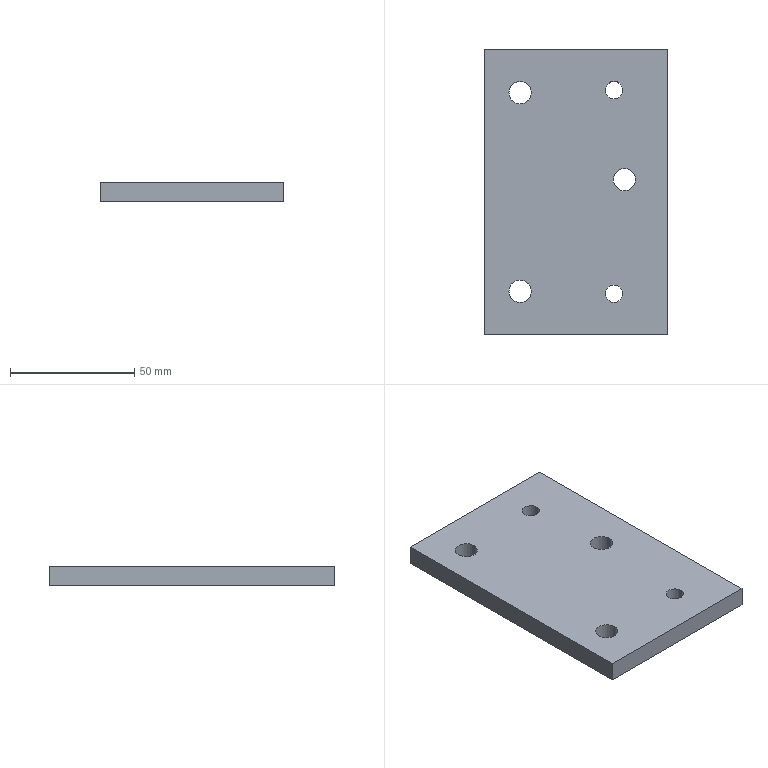Part | 1 solid | 16 faces | box 74 x 115 x 8 mm | volume 65938 mm3 | cylinder 10 | plane 6 | commonest cylinder face diameters 9 x6 7 x4
STEP:
#1=CARTESIAN_POINT('',(0.,0.,0.));
#2=DIRECTION('',(0.,0.,1.));
#3=DIRECTION('',(1.,0.,0.));
#4=AXIS2_PLACEMENT_3D('',#1,#2,#3);
#5=CARTESIAN_POINT('',(-185.5,244.,-105.051));
#6=VERTEX_POINT('',#5);
#7=CARTESIAN_POINT('',(-259.5,244.,-105.051));
#8=VERTEX_POINT('',#7);
#9=CARTESIAN_POINT('',(-185.5,244.,-105.051));
#10=DIRECTION('',(-1.,0.,0.));
#11=VECTOR('',#10,1.);
#12=LINE('',#9,#11);
#13=CARTESIAN_POINT('',(-185.5,244.,-113.051));
#14=DIRECTION('',(0.,1.,0.));
#15=DIRECTION('',(0.,0.,-1.));
#16=AXIS2_PLACEMENT_3D('',#13,#14,#15);
#17=PLANE('',#16);
#18=CARTESIAN_POINT('',(-8.,0.));
#19=DIRECTION('',(0.,1.));
#20=VECTOR('',#19,1.);
#21=LINE('',#18,#20);
#22=(GEOMETRIC_REPRESENTATION_CONTEXT(2)PARAMETRIC_REPRESENTATION_CONTEXT()REPRESENTATION_CONTEXT('',''));
#23=DEFINITIONAL_REPRESENTATION('',(#21),#22);
#24=PCURVE('',#17,#23);
#25=CARTESIAN_POINT('',(-207.188,260.5,-105.051));
#26=DIRECTION('',(0.,0.,1.));
#27=DIRECTION('',(-1.,0.,0.));
#28=AXIS2_PLACEMENT_3D('',#25,#26,#27);
#29=PLANE('',#28);
#30=CARTESIAN_POINT('',(-21.688,16.5));
#31=DIRECTION('',(1.,0.));
#32=VECTOR('',#31,1.);
#33=LINE('',#30,#32);
#34=(GEOMETRIC_REPRESENTATION_CONTEXT(2)PARAMETRIC_REPRESENTATION_CONTEXT()REPRESENTATION_CONTEXT('',''));
#35=DEFINITIONAL_REPRESENTATION('',(#33),#34);
#36=PCURVE('',#29,#35);
#37=SURFACE_CURVE('',#12,(#24,#36),.PCURVE_S1.);
#38=EDGE_CURVE('',#6,#8,#37,.T.);
#39=ORIENTED_EDGE('',*,*,#38,.T.);
#40=CARTESIAN_POINT('',(-259.5,244.,-113.051));
#41=VERTEX_POINT('',#40);
#42=CARTESIAN_POINT('',(-259.5,244.,-113.051));
#43=DIRECTION('',(0.,0.,1.));
#44=VECTOR('',#43,1.);
#45=LINE('',#42,#44);
#46=CARTESIAN_POINT('',(0.,74.));
#47=DIRECTION('',(-1.,0.));
#48=VECTOR('',#47,1.);
#49=LINE('',#46,#48);
#50=(GEOMETRIC_REPRESENTATION_CONTEXT(2)PARAMETRIC_REPRESENTATION_CONTEXT()REPRESENTATION_CONTEXT('',''));
#51=DEFINITIONAL_REPRESENTATION('',(#49),#50);
#52=PCURVE('',#17,#51);
#53=CARTESIAN_POINT('',(-259.5,244.,-113.051));
#54=DIRECTION('',(1.,0.,0.));
#55=DIRECTION('',(0.,0.,1.));
#56=AXIS2_PLACEMENT_3D('',#53,#54,#55);
#57=PLANE('',#56);
#58=CARTESIAN_POINT('',(0.,0.));
#59=DIRECTION('',(1.,0.));
#60=VECTOR('',#59,1.);
#61=LINE('',#58,#60);
#62=(GEOMETRIC_REPRESENTATION_CONTEXT(2)PARAMETRIC_REPRESENTATION_CONTEXT()REPRESENTATION_CONTEXT('',''));
#63=DEFINITIONAL_REPRESENTATION('',(#61),#62);
#64=PCURVE('',#57,#63);
#65=SURFACE_CURVE('',#45,(#52,#64),.PCURVE_S1.);
#66=EDGE_CURVE('',#41,#8,#65,.T.);
#67=ORIENTED_EDGE('',*,*,#66,.F.);
#68=CARTESIAN_POINT('',(-185.5,244.,-113.051));
#69=VERTEX_POINT('',#68);
#70=CARTESIAN_POINT('',(-185.5,244.,-113.051));
#71=DIRECTION('',(-1.,0.,0.));
#72=VECTOR('',#71,1.);
#73=LINE('',#70,#72);
#74=CARTESIAN_POINT('',(0.,0.));
#75=DIRECTION('',(0.,1.));
#76=VECTOR('',#75,1.);
#77=LINE('',#74,#76);
#78=(GEOMETRIC_REPRESENTATION_CONTEXT(2)PARAMETRIC_REPRESENTATION_CONTEXT()REPRESENTATION_CONTEXT('',''));
#79=DEFINITIONAL_REPRESENTATION('',(#77),#78);
#80=PCURVE('',#17,#79);
#81=CARTESIAN_POINT('',(-207.188,260.5,-113.051));
#82=DIRECTION('',(0.,0.,1.));
#83=DIRECTION('',(-1.,0.,0.));
#84=AXIS2_PLACEMENT_3D('',#81,#82,#83);
#85=PLANE('',#84);
#86=CARTESIAN_POINT('',(-21.688,16.5));
#87=DIRECTION('',(1.,0.));
#88=VECTOR('',#87,1.);
#89=LINE('',#86,#88);
#90=(GEOMETRIC_REPRESENTATION_CONTEXT(2)PARAMETRIC_REPRESENTATION_CONTEXT()REPRESENTATION_CONTEXT('',''));
#91=DEFINITIONAL_REPRESENTATION('',(#89),#90);
#92=PCURVE('',#85,#91);
#93=SURFACE_CURVE('',#73,(#80,#92),.PCURVE_S1.);
#94=EDGE_CURVE('',#69,#41,#93,.T.);
#95=ORIENTED_EDGE('',*,*,#94,.F.);
#96=CARTESIAN_POINT('',(-185.5,244.,-113.051));
#97=DIRECTION('',(0.,0.,1.));
#98=VECTOR('',#97,1.);
#99=LINE('',#96,#98);
#100=CARTESIAN_POINT('',(0.,0.));
#101=DIRECTION('',(-1.,0.));
#102=VECTOR('',#101,1.);
#103=LINE('',#100,#102);
#104=(GEOMETRIC_REPRESENTATION_CONTEXT(2)PARAMETRIC_REPRESENTATION_CONTEXT()REPRESENTATION_CONTEXT('',''));
#105=DEFINITIONAL_REPRESENTATION('',(#103),#104);
#106=PCURVE('',#17,#105);
#107=CARTESIAN_POINT('',(-185.5,359.,-113.051));
#108=DIRECTION('',(-1.,0.,0.));
#109=DIRECTION('',(0.,0.,-1.));
#110=AXIS2_PLACEMENT_3D('',#107,#108,#109);
#111=PLANE('',#110);
#112=CARTESIAN_POINT('',(0.,115.));
#113=DIRECTION('',(-1.,0.));
#114=VECTOR('',#113,1.);
#115=LINE('',#112,#114);
#116=(GEOMETRIC_REPRESENTATION_CONTEXT(2)PARAMETRIC_REPRESENTATION_CONTEXT()REPRESENTATION_CONTEXT('',''));
#117=DEFINITIONAL_REPRESENTATION('',(#115),#116);
#118=PCURVE('',#111,#117);
#119=SURFACE_CURVE('',#99,(#106,#118),.PCURVE_S1.);
#120=EDGE_CURVE('',#69,#6,#119,.T.);
#121=ORIENTED_EDGE('',*,*,#120,.T.);
#122=EDGE_LOOP('',(#39,#67,#95,#121));
#123=FACE_BOUND('',#122,.T.);
#124=ADVANCED_FACE('',(#123),#17,.F.);
#125=CARTESIAN_POINT('',(-185.5,359.,-105.051));
#126=VERTEX_POINT('',#125);
#127=CARTESIAN_POINT('',(-185.5,359.,-105.051));
#128=DIRECTION('',(0.,-1.,0.));
#129=VECTOR('',#128,1.);
#130=LINE('',#127,#129);
#131=CARTESIAN_POINT('',(-8.,0.));
#132=DIRECTION('',(0.,1.));
#133=VECTOR('',#132,1.);
#134=LINE('',#131,#133);
#135=(GEOMETRIC_REPRESENTATION_CONTEXT(2)PARAMETRIC_REPRESENTATION_CONTEXT()REPRESENTATION_CONTEXT('',''));
#136=DEFINITIONAL_REPRESENTATION('',(#134),#135);
#137=PCURVE('',#111,#136);
#138=CARTESIAN_POINT('',(-21.688,-98.5));
#139=DIRECTION('',(0.,1.));
#140=VECTOR('',#139,1.);
#141=LINE('',#138,#140);
#142=(GEOMETRIC_REPRESENTATION_CONTEXT(2)PARAMETRIC_REPRESENTATION_CONTEXT()REPRESENTATION_CONTEXT('',''));
#143=DEFINITIONAL_REPRESENTATION('',(#141),#142);
#144=PCURVE('',#29,#143);
#145=SURFACE_CURVE('',#130,(#137,#144),.PCURVE_S1.);
#146=EDGE_CURVE('',#126,#6,#145,.T.);
#147=ORIENTED_EDGE('',*,*,#146,.T.);
#148=ORIENTED_EDGE('',*,*,#120,.F.);
#149=CARTESIAN_POINT('',(-185.5,359.,-113.051));
#150=VERTEX_POINT('',#149);
#151=CARTESIAN_POINT('',(-185.5,359.,-113.051));
#152=DIRECTION('',(0.,-1.,0.));
#153=VECTOR('',#152,1.);
#154=LINE('',#151,#153);
#155=CARTESIAN_POINT('',(0.,0.));
#156=DIRECTION('',(0.,1.));
#157=VECTOR('',#156,1.);
#158=LINE('',#155,#157);
#159=(GEOMETRIC_REPRESENTATION_CONTEXT(2)PARAMETRIC_REPRESENTATION_CONTEXT()REPRESENTATION_CONTEXT('',''));
#160=DEFINITIONAL_REPRESENTATION('',(#158),#159);
#161=PCURVE('',#111,#160);
#162=CARTESIAN_POINT('',(-21.688,-98.5));
#163=DIRECTION('',(0.,1.));
#164=VECTOR('',#163,1.);
#165=LINE('',#162,#164);
#166=(GEOMETRIC_REPRESENTATION_CONTEXT(2)PARAMETRIC_REPRESENTATION_CONTEXT()REPRESENTATION_CONTEXT('',''));
#167=DEFINITIONAL_REPRESENTATION('',(#165),#166);
#168=PCURVE('',#85,#167);
#169=SURFACE_CURVE('',#154,(#161,#168),.PCURVE_S1.);
#170=EDGE_CURVE('',#150,#69,#169,.T.);
#171=ORIENTED_EDGE('',*,*,#170,.F.);
#172=CARTESIAN_POINT('',(-185.5,359.,-113.051));
#173=DIRECTION('',(0.,0.,1.));
#174=VECTOR('',#173,1.);
#175=LINE('',#172,#174);
#176=CARTESIAN_POINT('',(0.,0.));
#177=DIRECTION('',(-1.,0.));
#178=VECTOR('',#177,1.);
#179=LINE('',#176,#178);
#180=(GEOMETRIC_REPRESENTATION_CONTEXT(2)PARAMETRIC_REPRESENTATION_CONTEXT()REPRESENTATION_CONTEXT('',''));
#181=DEFINITIONAL_REPRESENTATION('',(#179),#180);
#182=PCURVE('',#111,#181);
#183=CARTESIAN_POINT('',(-259.5,359.,-113.051));
#184=DIRECTION('',(0.,-1.,0.));
#185=DIRECTION('',(0.,0.,1.));
#186=AXIS2_PLACEMENT_3D('',#183,#184,#185);
#187=PLANE('',#186);
#188=CARTESIAN_POINT('',(0.,-74.));
#189=DIRECTION('',(1.,0.));
#190=VECTOR('',#189,1.);
#191=LINE('',#188,#190);
#192=(GEOMETRIC_REPRESENTATION_CONTEXT(2)PARAMETRIC_REPRESENTATION_CONTEXT()REPRESENTATION_CONTEXT('',''));
#193=DEFINITIONAL_REPRESENTATION('',(#191),#192);
#194=PCURVE('',#187,#193);
#195=SURFACE_CURVE('',#175,(#182,#194),.PCURVE_S1.);
#196=EDGE_CURVE('',#150,#126,#195,.T.);
#197=ORIENTED_EDGE('',*,*,#196,.T.);
#198=EDGE_LOOP('',(#147,#148,#171,#197));
#199=FACE_BOUND('',#198,.T.);
#200=ADVANCED_FACE('',(#199),#111,.F.);
#201=CARTESIAN_POINT('',(-259.5,359.,-105.051));
#202=VERTEX_POINT('',#201);
#203=CARTESIAN_POINT('',(-259.5,359.,-105.051));
#204=DIRECTION('',(1.,0.,0.));
#205=VECTOR('',#204,1.);
#206=LINE('',#203,#205);
#207=CARTESIAN_POINT('',(8.,0.));
#208=DIRECTION('',(0.,-1.));
#209=VECTOR('',#208,1.);
#210=LINE('',#207,#209);
#211=(GEOMETRIC_REPRESENTATION_CONTEXT(2)PARAMETRIC_REPRESENTATION_CONTEXT()REPRESENTATION_CONTEXT('',''));
#212=DEFINITIONAL_REPRESENTATION('',(#210),#211);
#213=PCURVE('',#187,#212);
#214=CARTESIAN_POINT('',(52.312,-98.5));
#215=DIRECTION('',(-1.,0.));
#216=VECTOR('',#215,1.);
#217=LINE('',#214,#216);
#218=(GEOMETRIC_REPRESENTATION_CONTEXT(2)PARAMETRIC_REPRESENTATION_CONTEXT()REPRESENTATION_CONTEXT('',''));
#219=DEFINITIONAL_REPRESENTATION('',(#217),#218);
#220=PCURVE('',#29,#219);
#221=SURFACE_CURVE('',#206,(#213,#220),.PCURVE_S1.);
#222=EDGE_CURVE('',#202,#126,#221,.T.);
#223=ORIENTED_EDGE('',*,*,#222,.T.);
#224=ORIENTED_EDGE('',*,*,#196,.F.);
#225=CARTESIAN_POINT('',(-259.5,359.,-113.051));
#226=VERTEX_POINT('',#225);
#227=CARTESIAN_POINT('',(-259.5,359.,-113.051));
#228=DIRECTION('',(1.,0.,0.));
#229=VECTOR('',#228,1.);
#230=LINE('',#227,#229);
#231=CARTESIAN_POINT('',(0.,0.));
#232=DIRECTION('',(0.,-1.));
#233=VECTOR('',#232,1.);
#234=LINE('',#231,#233);
#235=(GEOMETRIC_REPRESENTATION_CONTEXT(2)PARAMETRIC_REPRESENTATION_CONTEXT()REPRESENTATION_CONTEXT('',''));
#236=DEFINITIONAL_REPRESENTATION('',(#234),#235);
#237=PCURVE('',#187,#236);
#238=CARTESIAN_POINT('',(52.312,-98.5));
#239=DIRECTION('',(-1.,0.));
#240=VECTOR('',#239,1.);
#241=LINE('',#238,#240);
#242=(GEOMETRIC_REPRESENTATION_CONTEXT(2)PARAMETRIC_REPRESENTATION_CONTEXT()REPRESENTATION_CONTEXT('',''));
#243=DEFINITIONAL_REPRESENTATION('',(#241),#242);
#244=PCURVE('',#85,#243);
#245=SURFACE_CURVE('',#230,(#237,#244),.PCURVE_S1.);
#246=EDGE_CURVE('',#226,#150,#245,.T.);
#247=ORIENTED_EDGE('',*,*,#246,.F.);
#248=CARTESIAN_POINT('',(-259.5,359.,-113.051));
#249=DIRECTION('',(0.,0.,1.));
#250=VECTOR('',#249,1.);
#251=LINE('',#248,#250);
#252=CARTESIAN_POINT('',(0.,0.));
#253=DIRECTION('',(1.,0.));
#254=VECTOR('',#253,1.);
#255=LINE('',#252,#254);
#256=(GEOMETRIC_REPRESENTATION_CONTEXT(2)PARAMETRIC_REPRESENTATION_CONTEXT()REPRESENTATION_CONTEXT('',''));
#257=DEFINITIONAL_REPRESENTATION('',(#255),#256);
#258=PCURVE('',#187,#257);
#259=CARTESIAN_POINT('',(0.,-115.));
#260=DIRECTION('',(1.,0.));
#261=VECTOR('',#260,1.);
#262=LINE('',#259,#261);
#263=(GEOMETRIC_REPRESENTATION_CONTEXT(2)PARAMETRIC_REPRESENTATION_CONTEXT()REPRESENTATION_CONTEXT('',''));
#264=DEFINITIONAL_REPRESENTATION('',(#262),#263);
#265=PCURVE('',#57,#264);
#266=SURFACE_CURVE('',#251,(#258,#265),.PCURVE_S1.);
#267=EDGE_CURVE('',#226,#202,#266,.T.);
#268=ORIENTED_EDGE('',*,*,#267,.T.);
#269=EDGE_LOOP('',(#223,#224,#247,#268));
#270=FACE_BOUND('',#269,.T.);
#271=ADVANCED_FACE('',(#270),#187,.F.);
#272=CARTESIAN_POINT('',(-259.5,244.,-105.051));
#273=DIRECTION('',(0.,1.,0.));
#274=VECTOR('',#273,1.);
#275=LINE('',#272,#274);
#276=CARTESIAN_POINT('',(8.,0.));
#277=DIRECTION('',(0.,-1.));
#278=VECTOR('',#277,1.);
#279=LINE('',#276,#278);
#280=(GEOMETRIC_REPRESENTATION_CONTEXT(2)PARAMETRIC_REPRESENTATION_CONTEXT()REPRESENTATION_CONTEXT('',''));
#281=DEFINITIONAL_REPRESENTATION('',(#279),#280);
#282=PCURVE('',#57,#281);
#283=CARTESIAN_POINT('',(52.312,16.5));
#284=DIRECTION('',(0.,-1.));
#285=VECTOR('',#284,1.);
#286=LINE('',#283,#285);
#287=(GEOMETRIC_REPRESENTATION_CONTEXT(2)PARAMETRIC_REPRESENTATION_CONTEXT()REPRESENTATION_CONTEXT('',''));
#288=DEFINITIONAL_REPRESENTATION('',(#286),#287);
#289=PCURVE('',#29,#288);
#290=SURFACE_CURVE('',#275,(#282,#289),.PCURVE_S1.);
#291=EDGE_CURVE('',#8,#202,#290,.T.);
#292=ORIENTED_EDGE('',*,*,#291,.T.);
#293=ORIENTED_EDGE('',*,*,#267,.F.);
#294=CARTESIAN_POINT('',(-259.5,244.,-113.051));
#295=DIRECTION('',(0.,1.,0.));
#296=VECTOR('',#295,1.);
#297=LINE('',#294,#296);
#298=CARTESIAN_POINT('',(0.,0.));
#299=DIRECTION('',(0.,-1.));
#300=VECTOR('',#299,1.);
#301=LINE('',#298,#300);
#302=(GEOMETRIC_REPRESENTATION_CONTEXT(2)PARAMETRIC_REPRESENTATION_CONTEXT()REPRESENTATION_CONTEXT('',''));
#303=DEFINITIONAL_REPRESENTATION('',(#301),#302);
#304=PCURVE('',#57,#303);
#305=CARTESIAN_POINT('',(52.312,16.5));
#306=DIRECTION('',(0.,-1.));
#307=VECTOR('',#306,1.);
#308=LINE('',#305,#307);
#309=(GEOMETRIC_REPRESENTATION_CONTEXT(2)PARAMETRIC_REPRESENTATION_CONTEXT()REPRESENTATION_CONTEXT('',''));
#310=DEFINITIONAL_REPRESENTATION('',(#308),#309);
#311=PCURVE('',#85,#310);
#312=SURFACE_CURVE('',#297,(#304,#311),.PCURVE_S1.);
#313=EDGE_CURVE('',#41,#226,#312,.T.);
#314=ORIENTED_EDGE('',*,*,#313,.F.);
#315=ORIENTED_EDGE('',*,*,#66,.T.);
#316=EDGE_LOOP('',(#292,#293,#314,#315));
#317=FACE_BOUND('',#316,.T.);
#318=ADVANCED_FACE('',(#317),#57,.F.);
#319=ORIENTED_EDGE('',*,*,#94,.T.);
#320=ORIENTED_EDGE('',*,*,#313,.T.);
#321=ORIENTED_EDGE('',*,*,#246,.T.);
#322=ORIENTED_EDGE('',*,*,#170,.T.);
#323=EDGE_LOOP('',(#319,#320,#321,#322));
#324=FACE_BOUND('',#323,.T.);
#325=CARTESIAN_POINT('',(-210.688,260.5,-113.051));
#326=VERTEX_POINT('',#325);
#327=CARTESIAN_POINT('',(-203.688,260.5,-113.051));
#328=VERTEX_POINT('',#327);
#329=CARTESIAN_POINT('',(-207.188,260.5,-113.051));
#330=DIRECTION('',(0.,0.,1.));
#331=DIRECTION('',(-1.,0.,0.));
#332=AXIS2_PLACEMENT_3D('',#329,#330,#331);
#333=CIRCLE('',#332,3.5);
#334=CARTESIAN_POINT('',(0.,0.));
#335=DIRECTION('',(1.,0.));
#336=AXIS2_PLACEMENT_2D('',#334,#335);
#337=CIRCLE('',#336,3.5);
#338=(GEOMETRIC_REPRESENTATION_CONTEXT(2)PARAMETRIC_REPRESENTATION_CONTEXT()REPRESENTATION_CONTEXT('',''));
#339=DEFINITIONAL_REPRESENTATION('',(#337),#338);
#340=PCURVE('',#85,#339);
#341=CARTESIAN_POINT('',(-207.188,260.5,-113.051));
#342=DIRECTION('',(0.,0.,1.));
#343=DIRECTION('',(0.,1.,0.));
#344=AXIS2_PLACEMENT_3D('',#341,#342,#343);
#345=CYLINDRICAL_SURFACE('',#344,3.5);
#346=CARTESIAN_POINT('',(1.571,0.));
#347=DIRECTION('',(1.,0.));
#348=VECTOR('',#347,1.);
#349=LINE('',#346,#348);
#350=(GEOMETRIC_REPRESENTATION_CONTEXT(2)PARAMETRIC_REPRESENTATION_CONTEXT()REPRESENTATION_CONTEXT('',''));
#351=DEFINITIONAL_REPRESENTATION('',(#349),#350);
#352=PCURVE('',#345,#351);
#353=SURFACE_CURVE('',#333,(#340,#352),.PCURVE_S1.);
#354=EDGE_CURVE('',#326,#328,#353,.T.);
#355=ORIENTED_EDGE('',*,*,#354,.T.);
#356=CARTESIAN_POINT('',(-207.188,260.5,-113.051));
#357=DIRECTION('',(0.,0.,1.));
#358=DIRECTION('',(-1.,0.,0.));
#359=AXIS2_PLACEMENT_3D('',#356,#357,#358);
#360=CIRCLE('',#359,3.5);
#361=CARTESIAN_POINT('',(0.,0.));
#362=DIRECTION('',(1.,0.));
#363=AXIS2_PLACEMENT_2D('',#361,#362);
#364=CIRCLE('',#363,3.5);
#365=(GEOMETRIC_REPRESENTATION_CONTEXT(2)PARAMETRIC_REPRESENTATION_CONTEXT()REPRESENTATION_CONTEXT('',''));
#366=DEFINITIONAL_REPRESENTATION('',(#364),#365);
#367=PCURVE('',#85,#366);
#368=CARTESIAN_POINT('',(-207.188,260.5,-113.051));
#369=DIRECTION('',(0.,0.,1.));
#370=DIRECTION('',(0.,-1.,0.));
#371=AXIS2_PLACEMENT_3D('',#368,#369,#370);
#372=CYLINDRICAL_SURFACE('',#371,3.5);
#373=CARTESIAN_POINT('',(-1.571,0.));
#374=DIRECTION('',(1.,0.));
#375=VECTOR('',#374,1.);
#376=LINE('',#373,#375);
#377=(GEOMETRIC_REPRESENTATION_CONTEXT(2)PARAMETRIC_REPRESENTATION_CONTEXT()REPRESENTATION_CONTEXT('',''));
#378=DEFINITIONAL_REPRESENTATION('',(#376),#377);
#379=PCURVE('',#372,#378);
#380=SURFACE_CURVE('',#360,(#367,#379),.PCURVE_S1.);
#381=EDGE_CURVE('',#328,#326,#380,.T.);
#382=ORIENTED_EDGE('',*,*,#381,.T.);
#383=EDGE_LOOP('',(#355,#382));
#384=FACE_BOUND('',#383,.T.);
#385=CARTESIAN_POINT('',(-207.5,306.5,-113.051));
#386=VERTEX_POINT('',#385);
#387=CARTESIAN_POINT('',(-198.5,306.5,-113.051));
#388=VERTEX_POINT('',#387);
#389=CARTESIAN_POINT('',(-203.,306.5,-113.051));
#390=DIRECTION('',(0.,0.,1.));
#391=DIRECTION('',(-1.,0.,0.));
#392=AXIS2_PLACEMENT_3D('',#389,#390,#391);
#393=CIRCLE('',#392,4.5);
#394=CARTESIAN_POINT('',(-4.188,-46.));
#395=DIRECTION('',(1.,0.));
#396=AXIS2_PLACEMENT_2D('',#394,#395);
#397=CIRCLE('',#396,4.5);
#398=(GEOMETRIC_REPRESENTATION_CONTEXT(2)PARAMETRIC_REPRESENTATION_CONTEXT()REPRESENTATION_CONTEXT('',''));
#399=DEFINITIONAL_REPRESENTATION('',(#397),#398);
#400=PCURVE('',#85,#399);
#401=CARTESIAN_POINT('',(-203.,306.5,-113.051));
#402=DIRECTION('',(0.,0.,1.));
#403=DIRECTION('',(0.,1.,0.));
#404=AXIS2_PLACEMENT_3D('',#401,#402,#403);
#405=CYLINDRICAL_SURFACE('',#404,4.5);
#406=CARTESIAN_POINT('',(1.571,0.));
#407=DIRECTION('',(1.,0.));
#408=VECTOR('',#407,1.);
#409=LINE('',#406,#408);
#410=(GEOMETRIC_REPRESENTATION_CONTEXT(2)PARAMETRIC_REPRESENTATION_CONTEXT()REPRESENTATION_CONTEXT('',''));
#411=DEFINITIONAL_REPRESENTATION('',(#409),#410);
#412=PCURVE('',#405,#411);
#413=SURFACE_CURVE('',#393,(#400,#412),.PCURVE_S1.);
#414=EDGE_CURVE('',#386,#388,#413,.T.);
#415=ORIENTED_EDGE('',*,*,#414,.T.);
#416=CARTESIAN_POINT('',(-203.,306.5,-113.051));
#417=DIRECTION('',(0.,0.,1.));
#418=DIRECTION('',(-1.,0.,0.));
#419=AXIS2_PLACEMENT_3D('',#416,#417,#418);
#420=CIRCLE('',#419,4.5);
#421=CARTESIAN_POINT('',(-4.188,-46.));
#422=DIRECTION('',(1.,0.));
#423=AXIS2_PLACEMENT_2D('',#421,#422);
#424=CIRCLE('',#423,4.5);
#425=(GEOMETRIC_REPRESENTATION_CONTEXT(2)PARAMETRIC_REPRESENTATION_CONTEXT()REPRESENTATION_CONTEXT('',''));
#426=DEFINITIONAL_REPRESENTATION('',(#424),#425);
#427=PCURVE('',#85,#426);
#428=CARTESIAN_POINT('',(-203.,306.5,-113.051));
#429=DIRECTION('',(0.,0.,1.));
#430=DIRECTION('',(0.,-1.,0.));
#431=AXIS2_PLACEMENT_3D('',#428,#429,#430);
#432=CYLINDRICAL_SURFACE('',#431,4.5);
#433=CARTESIAN_POINT('',(-1.571,0.));
#434=DIRECTION('',(1.,0.));
#435=VECTOR('',#434,1.);
#436=LINE('',#433,#435);
#437=(GEOMETRIC_REPRESENTATION_CONTEXT(2)PARAMETRIC_REPRESENTATION_CONTEXT()REPRESENTATION_CONTEXT('',''));
#438=DEFINITIONAL_REPRESENTATION('',(#436),#437);
#439=PCURVE('',#432,#438);
#440=SURFACE_CURVE('',#420,(#427,#439),.PCURVE_S1.);
#441=EDGE_CURVE('',#388,#386,#440,.T.);
#442=ORIENTED_EDGE('',*,*,#441,.T.);
#443=EDGE_LOOP('',(#415,#442));
#444=FACE_BOUND('',#443,.T.);
#445=CARTESIAN_POINT('',(-249.5,261.5,-113.051));
#446=VERTEX_POINT('',#445);
#447=CARTESIAN_POINT('',(-240.5,261.5,-113.051));
#448=VERTEX_POINT('',#447);
#449=CARTESIAN_POINT('',(-245.,261.5,-113.051));
#450=DIRECTION('',(0.,0.,1.));
#451=DIRECTION('',(-1.,0.,0.));
#452=AXIS2_PLACEMENT_3D('',#449,#450,#451);
#453=CIRCLE('',#452,4.5);
#454=CARTESIAN_POINT('',(37.812,-0.9999));
#455=DIRECTION('',(1.,0.));
#456=AXIS2_PLACEMENT_2D('',#454,#455);
#457=CIRCLE('',#456,4.5);
#458=(GEOMETRIC_REPRESENTATION_CONTEXT(2)PARAMETRIC_REPRESENTATION_CONTEXT()REPRESENTATION_CONTEXT('',''));
#459=DEFINITIONAL_REPRESENTATION('',(#457),#458);
#460=PCURVE('',#85,#459);
#461=CARTESIAN_POINT('',(-245.,261.5,-113.051));
#462=DIRECTION('',(0.,0.,1.));
#463=DIRECTION('',(0.,1.,0.));
#464=AXIS2_PLACEMENT_3D('',#461,#462,#463);
#465=CYLINDRICAL_SURFACE('',#464,4.5);
#466=CARTESIAN_POINT('',(1.571,0.));
#467=DIRECTION('',(1.,0.));
#468=VECTOR('',#467,1.);
#469=LINE('',#466,#468);
#470=(GEOMETRIC_REPRESENTATION_CONTEXT(2)PARAMETRIC_REPRESENTATION_CONTEXT()REPRESENTATION_CONTEXT('',''));
#471=DEFINITIONAL_REPRESENTATION('',(#469),#470);
#472=PCURVE('',#465,#471);
#473=SURFACE_CURVE('',#453,(#460,#472),.PCURVE_S1.);
#474=EDGE_CURVE('',#446,#448,#473,.T.);
#475=ORIENTED_EDGE('',*,*,#474,.T.);
#476=CARTESIAN_POINT('',(-245.,261.5,-113.051));
#477=DIRECTION('',(0.,0.,1.));
#478=DIRECTION('',(-1.,0.,0.));
#479=AXIS2_PLACEMENT_3D('',#476,#477,#478);
#480=CIRCLE('',#479,4.5);
#481=CARTESIAN_POINT('',(37.812,-0.9999));
#482=DIRECTION('',(1.,0.));
#483=AXIS2_PLACEMENT_2D('',#481,#482);
#484=CIRCLE('',#483,4.5);
#485=(GEOMETRIC_REPRESENTATION_CONTEXT(2)PARAMETRIC_REPRESENTATION_CONTEXT()REPRESENTATION_CONTEXT('',''));
#486=DEFINITIONAL_REPRESENTATION('',(#484),#485);
#487=PCURVE('',#85,#486);
#488=CARTESIAN_POINT('',(-245.,261.5,-113.051));
#489=DIRECTION('',(0.,0.,1.));
#490=DIRECTION('',(0.,-1.,0.));
#491=AXIS2_PLACEMENT_3D('',#488,#489,#490);
#492=CYLINDRICAL_SURFACE('',#491,4.5);
#493=CARTESIAN_POINT('',(-1.571,0.));
#494=DIRECTION('',(1.,0.));
#495=VECTOR('',#494,1.);
#496=LINE('',#493,#495);
#497=(GEOMETRIC_REPRESENTATION_CONTEXT(2)PARAMETRIC_REPRESENTATION_CONTEXT()REPRESENTATION_CONTEXT('',''));
#498=DEFINITIONAL_REPRESENTATION('',(#496),#497);
#499=PCURVE('',#492,#498);
#500=SURFACE_CURVE('',#480,(#487,#499),.PCURVE_S1.);
#501=EDGE_CURVE('',#448,#446,#500,.T.);
#502=ORIENTED_EDGE('',*,*,#501,.T.);
#503=EDGE_LOOP('',(#475,#502));
#504=FACE_BOUND('',#503,.T.);
#505=CARTESIAN_POINT('',(-210.688,342.5,-113.051));
#506=VERTEX_POINT('',#505);
#507=CARTESIAN_POINT('',(-203.688,342.5,-113.051));
#508=VERTEX_POINT('',#507);
#509=CARTESIAN_POINT('',(-207.188,342.5,-113.051));
#510=DIRECTION('',(0.,0.,1.));
#511=DIRECTION('',(-1.,0.,0.));
#512=AXIS2_PLACEMENT_3D('',#509,#510,#511);
#513=CIRCLE('',#512,3.5);
#514=CARTESIAN_POINT('',(0.,-82.));
#515=DIRECTION('',(1.,0.));
#516=AXIS2_PLACEMENT_2D('',#514,#515);
#517=CIRCLE('',#516,3.5);
#518=(GEOMETRIC_REPRESENTATION_CONTEXT(2)PARAMETRIC_REPRESENTATION_CONTEXT()REPRESENTATION_CONTEXT('',''));
#519=DEFINITIONAL_REPRESENTATION('',(#517),#518);
#520=PCURVE('',#85,#519);
#521=CARTESIAN_POINT('',(-207.188,342.5,-113.051));
#522=DIRECTION('',(0.,0.,1.));
#523=DIRECTION('',(0.,1.,0.));
#524=AXIS2_PLACEMENT_3D('',#521,#522,#523);
#525=CYLINDRICAL_SURFACE('',#524,3.5);
#526=CARTESIAN_POINT('',(1.571,0.));
#527=DIRECTION('',(1.,0.));
#528=VECTOR('',#527,1.);
#529=LINE('',#526,#528);
#530=(GEOMETRIC_REPRESENTATION_CONTEXT(2)PARAMETRIC_REPRESENTATION_CONTEXT()REPRESENTATION_CONTEXT('',''));
#531=DEFINITIONAL_REPRESENTATION('',(#529),#530);
#532=PCURVE('',#525,#531);
#533=SURFACE_CURVE('',#513,(#520,#532),.PCURVE_S1.);
#534=EDGE_CURVE('',#506,#508,#533,.T.);
#535=ORIENTED_EDGE('',*,*,#534,.T.);
#536=CARTESIAN_POINT('',(-207.188,342.5,-113.051));
#537=DIRECTION('',(0.,0.,1.));
#538=DIRECTION('',(-1.,0.,0.));
#539=AXIS2_PLACEMENT_3D('',#536,#537,#538);
#540=CIRCLE('',#539,3.5);
#541=CARTESIAN_POINT('',(0.,-82.));
#542=DIRECTION('',(1.,0.));
#543=AXIS2_PLACEMENT_2D('',#541,#542);
#544=CIRCLE('',#543,3.5);
#545=(GEOMETRIC_REPRESENTATION_CONTEXT(2)PARAMETRIC_REPRESENTATION_CONTEXT()REPRESENTATION_CONTEXT('',''));
#546=DEFINITIONAL_REPRESENTATION('',(#544),#545);
#547=PCURVE('',#85,#546);
#548=CARTESIAN_POINT('',(-207.188,342.5,-113.051));
#549=DIRECTION('',(0.,0.,1.));
#550=DIRECTION('',(0.,-1.,0.));
#551=AXIS2_PLACEMENT_3D('',#548,#549,#550);
#552=CYLINDRICAL_SURFACE('',#551,3.5);
#553=CARTESIAN_POINT('',(-1.571,0.));
#554=DIRECTION('',(1.,0.));
#555=VECTOR('',#554,1.);
#556=LINE('',#553,#555);
#557=(GEOMETRIC_REPRESENTATION_CONTEXT(2)PARAMETRIC_REPRESENTATION_CONTEXT()REPRESENTATION_CONTEXT('',''));
#558=DEFINITIONAL_REPRESENTATION('',(#556),#557);
#559=PCURVE('',#552,#558);
#560=SURFACE_CURVE('',#540,(#547,#559),.PCURVE_S1.);
#561=EDGE_CURVE('',#508,#506,#560,.T.);
#562=ORIENTED_EDGE('',*,*,#561,.T.);
#563=EDGE_LOOP('',(#535,#562));
#564=FACE_BOUND('',#563,.T.);
#565=CARTESIAN_POINT('',(-249.5,341.5,-113.051));
#566=VERTEX_POINT('',#565);
#567=CARTESIAN_POINT('',(-240.5,341.5,-113.051));
#568=VERTEX_POINT('',#567);
#569=CARTESIAN_POINT('',(-245.,341.5,-113.051));
#570=DIRECTION('',(0.,0.,1.));
#571=DIRECTION('',(-1.,0.,0.));
#572=AXIS2_PLACEMENT_3D('',#569,#570,#571);
#573=CIRCLE('',#572,4.5);
#574=CARTESIAN_POINT('',(37.812,-81.));
#575=DIRECTION('',(1.,0.));
#576=AXIS2_PLACEMENT_2D('',#574,#575);
#577=CIRCLE('',#576,4.5);
#578=(GEOMETRIC_REPRESENTATION_CONTEXT(2)PARAMETRIC_REPRESENTATION_CONTEXT()REPRESENTATION_CONTEXT('',''));
#579=DEFINITIONAL_REPRESENTATION('',(#577),#578);
#580=PCURVE('',#85,#579);
#581=CARTESIAN_POINT('',(-245.,341.5,-113.051));
#582=DIRECTION('',(0.,0.,1.));
#583=DIRECTION('',(0.,1.,0.));
#584=AXIS2_PLACEMENT_3D('',#581,#582,#583);
#585=CYLINDRICAL_SURFACE('',#584,4.5);
#586=CARTESIAN_POINT('',(1.571,0.));
#587=DIRECTION('',(1.,0.));
#588=VECTOR('',#587,1.);
#589=LINE('',#586,#588);
#590=(GEOMETRIC_REPRESENTATION_CONTEXT(2)PARAMETRIC_REPRESENTATION_CONTEXT()REPRESENTATION_CONTEXT('',''));
#591=DEFINITIONAL_REPRESENTATION('',(#589),#590);
#592=PCURVE('',#585,#591);
#593=SURFACE_CURVE('',#573,(#580,#592),.PCURVE_S1.);
#594=EDGE_CURVE('',#566,#568,#593,.T.);
#595=ORIENTED_EDGE('',*,*,#594,.T.);
#596=CARTESIAN_POINT('',(-245.,341.5,-113.051));
#597=DIRECTION('',(0.,0.,1.));
#598=DIRECTION('',(-1.,0.,0.));
#599=AXIS2_PLACEMENT_3D('',#596,#597,#598);
#600=CIRCLE('',#599,4.5);
#601=CARTESIAN_POINT('',(37.812,-81.));
#602=DIRECTION('',(1.,0.));
#603=AXIS2_PLACEMENT_2D('',#601,#602);
#604=CIRCLE('',#603,4.5);
#605=(GEOMETRIC_REPRESENTATION_CONTEXT(2)PARAMETRIC_REPRESENTATION_CONTEXT()REPRESENTATION_CONTEXT('',''));
#606=DEFINITIONAL_REPRESENTATION('',(#604),#605);
#607=PCURVE('',#85,#606);
#608=CARTESIAN_POINT('',(-245.,341.5,-113.051));
#609=DIRECTION('',(0.,0.,1.));
#610=DIRECTION('',(0.,-1.,0.));
#611=AXIS2_PLACEMENT_3D('',#608,#609,#610);
#612=CYLINDRICAL_SURFACE('',#611,4.5);
#613=CARTESIAN_POINT('',(-1.571,0.));
#614=DIRECTION('',(1.,0.));
#615=VECTOR('',#614,1.);
#616=LINE('',#613,#615);
#617=(GEOMETRIC_REPRESENTATION_CONTEXT(2)PARAMETRIC_REPRESENTATION_CONTEXT()REPRESENTATION_CONTEXT('',''));
#618=DEFINITIONAL_REPRESENTATION('',(#616),#617);
#619=PCURVE('',#612,#618);
#620=SURFACE_CURVE('',#600,(#607,#619),.PCURVE_S1.);
#621=EDGE_CURVE('',#568,#566,#620,.T.);
#622=ORIENTED_EDGE('',*,*,#621,.T.);
#623=EDGE_LOOP('',(#595,#622));
#624=FACE_BOUND('',#623,.T.);
#625=ADVANCED_FACE('',(#324,#384,#444,#504,#564,#624),#85,.F.);
#626=ORIENTED_EDGE('',*,*,#621,.T.);
#627=CARTESIAN_POINT('',(-249.5,341.5,-105.051));
#628=VERTEX_POINT('',#627);
#629=CARTESIAN_POINT('',(-249.5,341.5,-113.051));
#630=DIRECTION('',(0.,0.,1.));
#631=VECTOR('',#630,1.);
#632=LINE('',#629,#631);
#633=CARTESIAN_POINT('',(4.712,0.));
#634=DIRECTION('',(0.,1.));
#635=VECTOR('',#634,1.);
#636=LINE('',#633,#635);
#637=(GEOMETRIC_REPRESENTATION_CONTEXT(2)PARAMETRIC_REPRESENTATION_CONTEXT()REPRESENTATION_CONTEXT('',''));
#638=DEFINITIONAL_REPRESENTATION('',(#636),#637);
#639=PCURVE('',#612,#638);
#640=CARTESIAN_POINT('',(1.571,0.));
#641=DIRECTION('',(0.,1.));
#642=VECTOR('',#641,1.);
#643=LINE('',#640,#642);
#644=(GEOMETRIC_REPRESENTATION_CONTEXT(2)PARAMETRIC_REPRESENTATION_CONTEXT()REPRESENTATION_CONTEXT('',''));
#645=DEFINITIONAL_REPRESENTATION('',(#643),#644);
#646=PCURVE('',#585,#645);
#647=SURFACE_CURVE('',#632,(#639,#646),.PCURVE_S1.);
#648=EDGE_CURVE('',#566,#628,#647,.T.);
#649=ORIENTED_EDGE('',*,*,#648,.T.);
#650=CARTESIAN_POINT('',(-240.5,341.5,-105.051));
#651=VERTEX_POINT('',#650);
#652=CARTESIAN_POINT('',(-245.,341.5,-105.051));
#653=DIRECTION('',(0.,0.,1.));
#654=DIRECTION('',(-1.,0.,0.));
#655=AXIS2_PLACEMENT_3D('',#652,#653,#654);
#656=CIRCLE('',#655,4.5);
#657=CARTESIAN_POINT('',(-1.571,8.));
#658=DIRECTION('',(1.,0.));
#659=VECTOR('',#658,1.);
#660=LINE('',#657,#659);
#661=(GEOMETRIC_REPRESENTATION_CONTEXT(2)PARAMETRIC_REPRESENTATION_CONTEXT()REPRESENTATION_CONTEXT('',''));
#662=DEFINITIONAL_REPRESENTATION('',(#660),#661);
#663=PCURVE('',#612,#662);
#664=CARTESIAN_POINT('',(37.812,-81.));
#665=DIRECTION('',(1.,0.));
#666=AXIS2_PLACEMENT_2D('',#664,#665);
#667=CIRCLE('',#666,4.5);
#668=(GEOMETRIC_REPRESENTATION_CONTEXT(2)PARAMETRIC_REPRESENTATION_CONTEXT()REPRESENTATION_CONTEXT('',''));
#669=DEFINITIONAL_REPRESENTATION('',(#667),#668);
#670=PCURVE('',#29,#669);
#671=SURFACE_CURVE('',#656,(#663,#670),.PCURVE_S1.);
#672=EDGE_CURVE('',#651,#628,#671,.T.);
#673=ORIENTED_EDGE('',*,*,#672,.F.);
#674=CARTESIAN_POINT('',(-240.5,341.5,-113.051));
#675=DIRECTION('',(0.,0.,1.));
#676=VECTOR('',#675,1.);
#677=LINE('',#674,#676);
#678=CARTESIAN_POINT('',(1.571,0.));
#679=DIRECTION('',(0.,1.));
#680=VECTOR('',#679,1.);
#681=LINE('',#678,#680);
#682=(GEOMETRIC_REPRESENTATION_CONTEXT(2)PARAMETRIC_REPRESENTATION_CONTEXT()REPRESENTATION_CONTEXT('',''));
#683=DEFINITIONAL_REPRESENTATION('',(#681),#682);
#684=PCURVE('',#612,#683);
#685=CARTESIAN_POINT('',(4.712,0.));
#686=DIRECTION('',(0.,1.));
#687=VECTOR('',#686,1.);
#688=LINE('',#685,#687);
#689=(GEOMETRIC_REPRESENTATION_CONTEXT(2)PARAMETRIC_REPRESENTATION_CONTEXT()REPRESENTATION_CONTEXT('',''));
#690=DEFINITIONAL_REPRESENTATION('',(#688),#689);
#691=PCURVE('',#585,#690);
#692=SURFACE_CURVE('',#677,(#684,#691),.PCURVE_S1.);
#693=EDGE_CURVE('',#568,#651,#692,.T.);
#694=ORIENTED_EDGE('',*,*,#693,.F.);
#695=EDGE_LOOP('',(#626,#649,#673,#694));
#696=FACE_BOUND('',#695,.F.);
#697=ADVANCED_FACE('',(#696),#612,.F.);
#698=ORIENTED_EDGE('',*,*,#38,.F.);
#699=ORIENTED_EDGE('',*,*,#146,.F.);
#700=ORIENTED_EDGE('',*,*,#222,.F.);
#701=ORIENTED_EDGE('',*,*,#291,.F.);
#702=EDGE_LOOP('',(#698,#699,#700,#701));
#703=FACE_BOUND('',#702,.T.);
#704=CARTESIAN_POINT('',(-203.688,260.5,-105.051));
#705=VERTEX_POINT('',#704);
#706=CARTESIAN_POINT('',(-210.688,260.5,-105.051));
#707=VERTEX_POINT('',#706);
#708=CARTESIAN_POINT('',(-207.188,260.5,-105.051));
#709=DIRECTION('',(0.,0.,1.));
#710=DIRECTION('',(-1.,0.,0.));
#711=AXIS2_PLACEMENT_3D('',#708,#709,#710);
#712=CIRCLE('',#711,3.5);
#713=CARTESIAN_POINT('',(0.,0.));
#714=DIRECTION('',(1.,0.));
#715=AXIS2_PLACEMENT_2D('',#713,#714);
#716=CIRCLE('',#715,3.5);
#717=(GEOMETRIC_REPRESENTATION_CONTEXT(2)PARAMETRIC_REPRESENTATION_CONTEXT()REPRESENTATION_CONTEXT('',''));
#718=DEFINITIONAL_REPRESENTATION('',(#716),#717);
#719=PCURVE('',#29,#718);
#720=CARTESIAN_POINT('',(-1.571,8.));
#721=DIRECTION('',(1.,0.));
#722=VECTOR('',#721,1.);
#723=LINE('',#720,#722);
#724=(GEOMETRIC_REPRESENTATION_CONTEXT(2)PARAMETRIC_REPRESENTATION_CONTEXT()REPRESENTATION_CONTEXT('',''));
#725=DEFINITIONAL_REPRESENTATION('',(#723),#724);
#726=PCURVE('',#372,#725);
#727=SURFACE_CURVE('',#712,(#719,#726),.PCURVE_S1.);
#728=EDGE_CURVE('',#705,#707,#727,.T.);
#729=ORIENTED_EDGE('',*,*,#728,.F.);
#730=CARTESIAN_POINT('',(-207.188,260.5,-105.051));
#731=DIRECTION('',(0.,0.,1.));
#732=DIRECTION('',(-1.,0.,0.));
#733=AXIS2_PLACEMENT_3D('',#730,#731,#732);
#734=CIRCLE('',#733,3.5);
#735=CARTESIAN_POINT('',(0.,0.));
#736=DIRECTION('',(1.,0.));
#737=AXIS2_PLACEMENT_2D('',#735,#736);
#738=CIRCLE('',#737,3.5);
#739=(GEOMETRIC_REPRESENTATION_CONTEXT(2)PARAMETRIC_REPRESENTATION_CONTEXT()REPRESENTATION_CONTEXT('',''));
#740=DEFINITIONAL_REPRESENTATION('',(#738),#739);
#741=PCURVE('',#29,#740);
#742=CARTESIAN_POINT('',(1.571,8.));
#743=DIRECTION('',(1.,0.));
#744=VECTOR('',#743,1.);
#745=LINE('',#742,#744);
#746=(GEOMETRIC_REPRESENTATION_CONTEXT(2)PARAMETRIC_REPRESENTATION_CONTEXT()REPRESENTATION_CONTEXT('',''));
#747=DEFINITIONAL_REPRESENTATION('',(#745),#746);
#748=PCURVE('',#345,#747);
#749=SURFACE_CURVE('',#734,(#741,#748),.PCURVE_S1.);
#750=EDGE_CURVE('',#707,#705,#749,.T.);
#751=ORIENTED_EDGE('',*,*,#750,.F.);
#752=EDGE_LOOP('',(#729,#751));
#753=FACE_BOUND('',#752,.T.);
#754=CARTESIAN_POINT('',(-198.5,306.5,-105.051));
#755=VERTEX_POINT('',#754);
#756=CARTESIAN_POINT('',(-207.5,306.5,-105.051));
#757=VERTEX_POINT('',#756);
#758=CARTESIAN_POINT('',(-203.,306.5,-105.051));
#759=DIRECTION('',(0.,0.,1.));
#760=DIRECTION('',(-1.,0.,0.));
#761=AXIS2_PLACEMENT_3D('',#758,#759,#760);
#762=CIRCLE('',#761,4.5);
#763=CARTESIAN_POINT('',(-4.188,-46.));
#764=DIRECTION('',(1.,0.));
#765=AXIS2_PLACEMENT_2D('',#763,#764);
#766=CIRCLE('',#765,4.5);
#767=(GEOMETRIC_REPRESENTATION_CONTEXT(2)PARAMETRIC_REPRESENTATION_CONTEXT()REPRESENTATION_CONTEXT('',''));
#768=DEFINITIONAL_REPRESENTATION('',(#766),#767);
#769=PCURVE('',#29,#768);
#770=CARTESIAN_POINT('',(-1.571,8.));
#771=DIRECTION('',(1.,0.));
#772=VECTOR('',#771,1.);
#773=LINE('',#770,#772);
#774=(GEOMETRIC_REPRESENTATION_CONTEXT(2)PARAMETRIC_REPRESENTATION_CONTEXT()REPRESENTATION_CONTEXT('',''));
#775=DEFINITIONAL_REPRESENTATION('',(#773),#774);
#776=PCURVE('',#432,#775);
#777=SURFACE_CURVE('',#762,(#769,#776),.PCURVE_S1.);
#778=EDGE_CURVE('',#755,#757,#777,.T.);
#779=ORIENTED_EDGE('',*,*,#778,.F.);
#780=CARTESIAN_POINT('',(-203.,306.5,-105.051));
#781=DIRECTION('',(0.,0.,1.));
#782=DIRECTION('',(-1.,0.,0.));
#783=AXIS2_PLACEMENT_3D('',#780,#781,#782);
#784=CIRCLE('',#783,4.5);
#785=CARTESIAN_POINT('',(-4.188,-46.));
#786=DIRECTION('',(1.,0.));
#787=AXIS2_PLACEMENT_2D('',#785,#786);
#788=CIRCLE('',#787,4.5);
#789=(GEOMETRIC_REPRESENTATION_CONTEXT(2)PARAMETRIC_REPRESENTATION_CONTEXT()REPRESENTATION_CONTEXT('',''));
#790=DEFINITIONAL_REPRESENTATION('',(#788),#789);
#791=PCURVE('',#29,#790);
#792=CARTESIAN_POINT('',(1.571,8.));
#793=DIRECTION('',(1.,0.));
#794=VECTOR('',#793,1.);
#795=LINE('',#792,#794);
#796=(GEOMETRIC_REPRESENTATION_CONTEXT(2)PARAMETRIC_REPRESENTATION_CONTEXT()REPRESENTATION_CONTEXT('',''));
#797=DEFINITIONAL_REPRESENTATION('',(#795),#796);
#798=PCURVE('',#405,#797);
#799=SURFACE_CURVE('',#784,(#791,#798),.PCURVE_S1.);
#800=EDGE_CURVE('',#757,#755,#799,.T.);
#801=ORIENTED_EDGE('',*,*,#800,.F.);
#802=EDGE_LOOP('',(#779,#801));
#803=FACE_BOUND('',#802,.T.);
#804=CARTESIAN_POINT('',(-240.5,261.5,-105.051));
#805=VERTEX_POINT('',#804);
#806=CARTESIAN_POINT('',(-249.5,261.5,-105.051));
#807=VERTEX_POINT('',#806);
#808=CARTESIAN_POINT('',(-245.,261.5,-105.051));
#809=DIRECTION('',(0.,0.,1.));
#810=DIRECTION('',(-1.,0.,0.));
#811=AXIS2_PLACEMENT_3D('',#808,#809,#810);
#812=CIRCLE('',#811,4.5);
#813=CARTESIAN_POINT('',(37.812,-0.9999));
#814=DIRECTION('',(1.,0.));
#815=AXIS2_PLACEMENT_2D('',#813,#814);
#816=CIRCLE('',#815,4.5);
#817=(GEOMETRIC_REPRESENTATION_CONTEXT(2)PARAMETRIC_REPRESENTATION_CONTEXT()REPRESENTATION_CONTEXT('',''));
#818=DEFINITIONAL_REPRESENTATION('',(#816),#817);
#819=PCURVE('',#29,#818);
#820=CARTESIAN_POINT('',(-1.571,8.));
#821=DIRECTION('',(1.,0.));
#822=VECTOR('',#821,1.);
#823=LINE('',#820,#822);
#824=(GEOMETRIC_REPRESENTATION_CONTEXT(2)PARAMETRIC_REPRESENTATION_CONTEXT()REPRESENTATION_CONTEXT('',''));
#825=DEFINITIONAL_REPRESENTATION('',(#823),#824);
#826=PCURVE('',#492,#825);
#827=SURFACE_CURVE('',#812,(#819,#826),.PCURVE_S1.);
#828=EDGE_CURVE('',#805,#807,#827,.T.);
#829=ORIENTED_EDGE('',*,*,#828,.F.);
#830=CARTESIAN_POINT('',(-245.,261.5,-105.051));
#831=DIRECTION('',(0.,0.,1.));
#832=DIRECTION('',(-1.,0.,0.));
#833=AXIS2_PLACEMENT_3D('',#830,#831,#832);
#834=CIRCLE('',#833,4.5);
#835=CARTESIAN_POINT('',(37.812,-0.9999));
#836=DIRECTION('',(1.,0.));
#837=AXIS2_PLACEMENT_2D('',#835,#836);
#838=CIRCLE('',#837,4.5);
#839=(GEOMETRIC_REPRESENTATION_CONTEXT(2)PARAMETRIC_REPRESENTATION_CONTEXT()REPRESENTATION_CONTEXT('',''));
#840=DEFINITIONAL_REPRESENTATION('',(#838),#839);
#841=PCURVE('',#29,#840);
#842=CARTESIAN_POINT('',(1.571,8.));
#843=DIRECTION('',(1.,0.));
#844=VECTOR('',#843,1.);
#845=LINE('',#842,#844);
#846=(GEOMETRIC_REPRESENTATION_CONTEXT(2)PARAMETRIC_REPRESENTATION_CONTEXT()REPRESENTATION_CONTEXT('',''));
#847=DEFINITIONAL_REPRESENTATION('',(#845),#846);
#848=PCURVE('',#465,#847);
#849=SURFACE_CURVE('',#834,(#841,#848),.PCURVE_S1.);
#850=EDGE_CURVE('',#807,#805,#849,.T.);
#851=ORIENTED_EDGE('',*,*,#850,.F.);
#852=EDGE_LOOP('',(#829,#851));
#853=FACE_BOUND('',#852,.T.);
#854=CARTESIAN_POINT('',(-203.688,342.5,-105.051));
#855=VERTEX_POINT('',#854);
#856=CARTESIAN_POINT('',(-210.688,342.5,-105.051));
#857=VERTEX_POINT('',#856);
#858=CARTESIAN_POINT('',(-207.188,342.5,-105.051));
#859=DIRECTION('',(0.,0.,1.));
#860=DIRECTION('',(-1.,0.,0.));
#861=AXIS2_PLACEMENT_3D('',#858,#859,#860);
#862=CIRCLE('',#861,3.5);
#863=CARTESIAN_POINT('',(0.,-82.));
#864=DIRECTION('',(1.,0.));
#865=AXIS2_PLACEMENT_2D('',#863,#864);
#866=CIRCLE('',#865,3.5);
#867=(GEOMETRIC_REPRESENTATION_CONTEXT(2)PARAMETRIC_REPRESENTATION_CONTEXT()REPRESENTATION_CONTEXT('',''));
#868=DEFINITIONAL_REPRESENTATION('',(#866),#867);
#869=PCURVE('',#29,#868);
#870=CARTESIAN_POINT('',(-1.571,8.));
#871=DIRECTION('',(1.,0.));
#872=VECTOR('',#871,1.);
#873=LINE('',#870,#872);
#874=(GEOMETRIC_REPRESENTATION_CONTEXT(2)PARAMETRIC_REPRESENTATION_CONTEXT()REPRESENTATION_CONTEXT('',''));
#875=DEFINITIONAL_REPRESENTATION('',(#873),#874);
#876=PCURVE('',#552,#875);
#877=SURFACE_CURVE('',#862,(#869,#876),.PCURVE_S1.);
#878=EDGE_CURVE('',#855,#857,#877,.T.);
#879=ORIENTED_EDGE('',*,*,#878,.F.);
#880=CARTESIAN_POINT('',(-207.188,342.5,-105.051));
#881=DIRECTION('',(0.,0.,1.));
#882=DIRECTION('',(-1.,0.,0.));
#883=AXIS2_PLACEMENT_3D('',#880,#881,#882);
#884=CIRCLE('',#883,3.5);
#885=CARTESIAN_POINT('',(0.,-82.));
#886=DIRECTION('',(1.,0.));
#887=AXIS2_PLACEMENT_2D('',#885,#886);
#888=CIRCLE('',#887,3.5);
#889=(GEOMETRIC_REPRESENTATION_CONTEXT(2)PARAMETRIC_REPRESENTATION_CONTEXT()REPRESENTATION_CONTEXT('',''));
#890=DEFINITIONAL_REPRESENTATION('',(#888),#889);
#891=PCURVE('',#29,#890);
#892=CARTESIAN_POINT('',(1.571,8.));
#893=DIRECTION('',(1.,0.));
#894=VECTOR('',#893,1.);
#895=LINE('',#892,#894);
#896=(GEOMETRIC_REPRESENTATION_CONTEXT(2)PARAMETRIC_REPRESENTATION_CONTEXT()REPRESENTATION_CONTEXT('',''));
#897=DEFINITIONAL_REPRESENTATION('',(#895),#896);
#898=PCURVE('',#525,#897);
#899=SURFACE_CURVE('',#884,(#891,#898),.PCURVE_S1.);
#900=EDGE_CURVE('',#857,#855,#899,.T.);
#901=ORIENTED_EDGE('',*,*,#900,.F.);
#902=EDGE_LOOP('',(#879,#901));
#903=FACE_BOUND('',#902,.T.);
#904=ORIENTED_EDGE('',*,*,#672,.F.);
#905=CARTESIAN_POINT('',(-245.,341.5,-105.051));
#906=DIRECTION('',(0.,0.,1.));
#907=DIRECTION('',(-1.,0.,0.));
#908=AXIS2_PLACEMENT_3D('',#905,#906,#907);
#909=CIRCLE('',#908,4.5);
#910=CARTESIAN_POINT('',(37.812,-81.));
#911=DIRECTION('',(1.,0.));
#912=AXIS2_PLACEMENT_2D('',#910,#911);
#913=CIRCLE('',#912,4.5);
#914=(GEOMETRIC_REPRESENTATION_CONTEXT(2)PARAMETRIC_REPRESENTATION_CONTEXT()REPRESENTATION_CONTEXT('',''));
#915=DEFINITIONAL_REPRESENTATION('',(#913),#914);
#916=PCURVE('',#29,#915);
#917=CARTESIAN_POINT('',(1.571,8.));
#918=DIRECTION('',(1.,0.));
#919=VECTOR('',#918,1.);
#920=LINE('',#917,#919);
#921=(GEOMETRIC_REPRESENTATION_CONTEXT(2)PARAMETRIC_REPRESENTATION_CONTEXT()REPRESENTATION_CONTEXT('',''));
#922=DEFINITIONAL_REPRESENTATION('',(#920),#921);
#923=PCURVE('',#585,#922);
#924=SURFACE_CURVE('',#909,(#916,#923),.PCURVE_S1.);
#925=EDGE_CURVE('',#628,#651,#924,.T.);
#926=ORIENTED_EDGE('',*,*,#925,.F.);
#927=EDGE_LOOP('',(#904,#926));
#928=FACE_BOUND('',#927,.T.);
#929=ADVANCED_FACE('',(#703,#753,#803,#853,#903,#928),#29,.T.);
#930=ORIENTED_EDGE('',*,*,#561,.T.);
#931=CARTESIAN_POINT('',(-210.688,342.5,-113.051));
#932=DIRECTION('',(0.,0.,1.));
#933=VECTOR('',#932,1.);
#934=LINE('',#931,#933);
#935=CARTESIAN_POINT('',(4.712,0.));
#936=DIRECTION('',(0.,1.));
#937=VECTOR('',#936,1.);
#938=LINE('',#935,#937);
#939=(GEOMETRIC_REPRESENTATION_CONTEXT(2)PARAMETRIC_REPRESENTATION_CONTEXT()REPRESENTATION_CONTEXT('',''));
#940=DEFINITIONAL_REPRESENTATION('',(#938),#939);
#941=PCURVE('',#552,#940);
#942=CARTESIAN_POINT('',(1.571,0.));
#943=DIRECTION('',(0.,1.));
#944=VECTOR('',#943,1.);
#945=LINE('',#942,#944);
#946=(GEOMETRIC_REPRESENTATION_CONTEXT(2)PARAMETRIC_REPRESENTATION_CONTEXT()REPRESENTATION_CONTEXT('',''));
#947=DEFINITIONAL_REPRESENTATION('',(#945),#946);
#948=PCURVE('',#525,#947);
#949=SURFACE_CURVE('',#934,(#941,#948),.PCURVE_S1.);
#950=EDGE_CURVE('',#506,#857,#949,.T.);
#951=ORIENTED_EDGE('',*,*,#950,.T.);
#952=ORIENTED_EDGE('',*,*,#878,.F.);
#953=CARTESIAN_POINT('',(-203.688,342.5,-113.051));
#954=DIRECTION('',(0.,0.,1.));
#955=VECTOR('',#954,1.);
#956=LINE('',#953,#955);
#957=CARTESIAN_POINT('',(1.571,0.));
#958=DIRECTION('',(0.,1.));
#959=VECTOR('',#958,1.);
#960=LINE('',#957,#959);
#961=(GEOMETRIC_REPRESENTATION_CONTEXT(2)PARAMETRIC_REPRESENTATION_CONTEXT()REPRESENTATION_CONTEXT('',''));
#962=DEFINITIONAL_REPRESENTATION('',(#960),#961);
#963=PCURVE('',#552,#962);
#964=CARTESIAN_POINT('',(4.712,0.));
#965=DIRECTION('',(0.,1.));
#966=VECTOR('',#965,1.);
#967=LINE('',#964,#966);
#968=(GEOMETRIC_REPRESENTATION_CONTEXT(2)PARAMETRIC_REPRESENTATION_CONTEXT()REPRESENTATION_CONTEXT('',''));
#969=DEFINITIONAL_REPRESENTATION('',(#967),#968);
#970=PCURVE('',#525,#969);
#971=SURFACE_CURVE('',#956,(#963,#970),.PCURVE_S1.);
#972=EDGE_CURVE('',#508,#855,#971,.T.);
#973=ORIENTED_EDGE('',*,*,#972,.F.);
#974=EDGE_LOOP('',(#930,#951,#952,#973));
#975=FACE_BOUND('',#974,.F.);
#976=ADVANCED_FACE('',(#975),#552,.F.);
#977=ORIENTED_EDGE('',*,*,#501,.T.);
#978=CARTESIAN_POINT('',(-249.5,261.5,-113.051));
#979=DIRECTION('',(0.,0.,1.));
#980=VECTOR('',#979,1.);
#981=LINE('',#978,#980);
#982=CARTESIAN_POINT('',(4.712,0.));
#983=DIRECTION('',(0.,1.));
#984=VECTOR('',#983,1.);
#985=LINE('',#982,#984);
#986=(GEOMETRIC_REPRESENTATION_CONTEXT(2)PARAMETRIC_REPRESENTATION_CONTEXT()REPRESENTATION_CONTEXT('',''));
#987=DEFINITIONAL_REPRESENTATION('',(#985),#986);
#988=PCURVE('',#492,#987);
#989=CARTESIAN_POINT('',(1.571,0.));
#990=DIRECTION('',(0.,1.));
#991=VECTOR('',#990,1.);
#992=LINE('',#989,#991);
#993=(GEOMETRIC_REPRESENTATION_CONTEXT(2)PARAMETRIC_REPRESENTATION_CONTEXT()REPRESENTATION_CONTEXT('',''));
#994=DEFINITIONAL_REPRESENTATION('',(#992),#993);
#995=PCURVE('',#465,#994);
#996=SURFACE_CURVE('',#981,(#988,#995),.PCURVE_S1.);
#997=EDGE_CURVE('',#446,#807,#996,.T.);
#998=ORIENTED_EDGE('',*,*,#997,.T.);
#999=ORIENTED_EDGE('',*,*,#828,.F.);
#1000=CARTESIAN_POINT('',(-240.5,261.5,-113.051));
#1001=DIRECTION('',(0.,0.,1.));
#1002=VECTOR('',#1001,1.);
#1003=LINE('',#1000,#1002);
#1004=CARTESIAN_POINT('',(1.571,0.));
#1005=DIRECTION('',(0.,1.));
#1006=VECTOR('',#1005,1.);
#1007=LINE('',#1004,#1006);
#1008=(GEOMETRIC_REPRESENTATION_CONTEXT(2)PARAMETRIC_REPRESENTATION_CONTEXT()REPRESENTATION_CONTEXT('',''));
#1009=DEFINITIONAL_REPRESENTATION('',(#1007),#1008);
#1010=PCURVE('',#492,#1009);
#1011=CARTESIAN_POINT('',(4.712,0.));
#1012=DIRECTION('',(0.,1.));
#1013=VECTOR('',#1012,1.);
#1014=LINE('',#1011,#1013);
#1015=(GEOMETRIC_REPRESENTATION_CONTEXT(2)PARAMETRIC_REPRESENTATION_CONTEXT()REPRESENTATION_CONTEXT('',''));
#1016=DEFINITIONAL_REPRESENTATION('',(#1014),#1015);
#1017=PCURVE('',#465,#1016);
#1018=SURFACE_CURVE('',#1003,(#1010,#1017),.PCURVE_S1.);
#1019=EDGE_CURVE('',#448,#805,#1018,.T.);
#1020=ORIENTED_EDGE('',*,*,#1019,.F.);
#1021=EDGE_LOOP('',(#977,#998,#999,#1020));
#1022=FACE_BOUND('',#1021,.F.);
#1023=ADVANCED_FACE('',(#1022),#492,.F.);
#1024=ORIENTED_EDGE('',*,*,#441,.T.);
#1025=CARTESIAN_POINT('',(-207.5,306.5,-113.051));
#1026=DIRECTION('',(0.,0.,1.));
#1027=VECTOR('',#1026,1.);
#1028=LINE('',#1025,#1027);
#1029=CARTESIAN_POINT('',(4.712,0.));
#1030=DIRECTION('',(0.,1.));
#1031=VECTOR('',#1030,1.);
#1032=LINE('',#1029,#1031);
#1033=(GEOMETRIC_REPRESENTATION_CONTEXT(2)PARAMETRIC_REPRESENTATION_CONTEXT()REPRESENTATION_CONTEXT('',''));
#1034=DEFINITIONAL_REPRESENTATION('',(#1032),#1033);
#1035=PCURVE('',#432,#1034);
#1036=CARTESIAN_POINT('',(1.571,0.));
#1037=DIRECTION('',(0.,1.));
#1038=VECTOR('',#1037,1.);
#1039=LINE('',#1036,#1038);
#1040=(GEOMETRIC_REPRESENTATION_CONTEXT(2)PARAMETRIC_REPRESENTATION_CONTEXT()REPRESENTATION_CONTEXT('',''));
#1041=DEFINITIONAL_REPRESENTATION('',(#1039),#1040);
#1042=PCURVE('',#405,#1041);
#1043=SURFACE_CURVE('',#1028,(#1035,#1042),.PCURVE_S1.);
#1044=EDGE_CURVE('',#386,#757,#1043,.T.);
#1045=ORIENTED_EDGE('',*,*,#1044,.T.);
#1046=ORIENTED_EDGE('',*,*,#778,.F.);
#1047=CARTESIAN_POINT('',(-198.5,306.5,-113.051));
#1048=DIRECTION('',(0.,0.,1.));
#1049=VECTOR('',#1048,1.);
#1050=LINE('',#1047,#1049);
#1051=CARTESIAN_POINT('',(1.571,0.));
#1052=DIRECTION('',(0.,1.));
#1053=VECTOR('',#1052,1.);
#1054=LINE('',#1051,#1053);
#1055=(GEOMETRIC_REPRESENTATION_CONTEXT(2)PARAMETRIC_REPRESENTATION_CONTEXT()REPRESENTATION_CONTEXT('',''));
#1056=DEFINITIONAL_REPRESENTATION('',(#1054),#1055);
#1057=PCURVE('',#432,#1056);
#1058=CARTESIAN_POINT('',(4.712,0.));
#1059=DIRECTION('',(0.,1.));
#1060=VECTOR('',#1059,1.);
#1061=LINE('',#1058,#1060);
#1062=(GEOMETRIC_REPRESENTATION_CONTEXT(2)PARAMETRIC_REPRESENTATION_CONTEXT()REPRESENTATION_CONTEXT('',''));
#1063=DEFINITIONAL_REPRESENTATION('',(#1061),#1062);
#1064=PCURVE('',#405,#1063);
#1065=SURFACE_CURVE('',#1050,(#1057,#1064),.PCURVE_S1.);
#1066=EDGE_CURVE('',#388,#755,#1065,.T.);
#1067=ORIENTED_EDGE('',*,*,#1066,.F.);
#1068=EDGE_LOOP('',(#1024,#1045,#1046,#1067));
#1069=FACE_BOUND('',#1068,.F.);
#1070=ADVANCED_FACE('',(#1069),#432,.F.);
#1071=ORIENTED_EDGE('',*,*,#381,.T.);
#1072=CARTESIAN_POINT('',(-210.688,260.5,-113.051));
#1073=DIRECTION('',(0.,0.,1.));
#1074=VECTOR('',#1073,1.);
#1075=LINE('',#1072,#1074);
#1076=CARTESIAN_POINT('',(4.712,0.));
#1077=DIRECTION('',(0.,1.));
#1078=VECTOR('',#1077,1.);
#1079=LINE('',#1076,#1078);
#1080=(GEOMETRIC_REPRESENTATION_CONTEXT(2)PARAMETRIC_REPRESENTATION_CONTEXT()REPRESENTATION_CONTEXT('',''));
#1081=DEFINITIONAL_REPRESENTATION('',(#1079),#1080);
#1082=PCURVE('',#372,#1081);
#1083=CARTESIAN_POINT('',(1.571,0.));
#1084=DIRECTION('',(0.,1.));
#1085=VECTOR('',#1084,1.);
#1086=LINE('',#1083,#1085);
#1087=(GEOMETRIC_REPRESENTATION_CONTEXT(2)PARAMETRIC_REPRESENTATION_CONTEXT()REPRESENTATION_CONTEXT('',''));
#1088=DEFINITIONAL_REPRESENTATION('',(#1086),#1087);
#1089=PCURVE('',#345,#1088);
#1090=SURFACE_CURVE('',#1075,(#1082,#1089),.PCURVE_S1.);
#1091=EDGE_CURVE('',#326,#707,#1090,.T.);
#1092=ORIENTED_EDGE('',*,*,#1091,.T.);
#1093=ORIENTED_EDGE('',*,*,#728,.F.);
#1094=CARTESIAN_POINT('',(-203.688,260.5,-113.051));
#1095=DIRECTION('',(0.,0.,1.));
#1096=VECTOR('',#1095,1.);
#1097=LINE('',#1094,#1096);
#1098=CARTESIAN_POINT('',(1.571,0.));
#1099=DIRECTION('',(0.,1.));
#1100=VECTOR('',#1099,1.);
#1101=LINE('',#1098,#1100);
#1102=(GEOMETRIC_REPRESENTATION_CONTEXT(2)PARAMETRIC_REPRESENTATION_CONTEXT()REPRESENTATION_CONTEXT('',''));
#1103=DEFINITIONAL_REPRESENTATION('',(#1101),#1102);
#1104=PCURVE('',#372,#1103);
#1105=CARTESIAN_POINT('',(4.712,0.));
#1106=DIRECTION('',(0.,1.));
#1107=VECTOR('',#1106,1.);
#1108=LINE('',#1105,#1107);
#1109=(GEOMETRIC_REPRESENTATION_CONTEXT(2)PARAMETRIC_REPRESENTATION_CONTEXT()REPRESENTATION_CONTEXT('',''));
#1110=DEFINITIONAL_REPRESENTATION('',(#1108),#1109);
#1111=PCURVE('',#345,#1110);
#1112=SURFACE_CURVE('',#1097,(#1104,#1111),.PCURVE_S1.);
#1113=EDGE_CURVE('',#328,#705,#1112,.T.);
#1114=ORIENTED_EDGE('',*,*,#1113,.F.);
#1115=EDGE_LOOP('',(#1071,#1092,#1093,#1114));
#1116=FACE_BOUND('',#1115,.F.);
#1117=ADVANCED_FACE('',(#1116),#372,.F.);
#1118=ORIENTED_EDGE('',*,*,#925,.F.);
#1119=ORIENTED_EDGE('',*,*,#648,.F.);
#1120=ORIENTED_EDGE('',*,*,#594,.T.);
#1121=ORIENTED_EDGE('',*,*,#693,.T.);
#1122=EDGE_LOOP('',(#1118,#1119,#1120,#1121));
#1123=FACE_BOUND('',#1122,.F.);
#1124=ADVANCED_FACE('',(#1123),#585,.F.);
#1125=ORIENTED_EDGE('',*,*,#900,.F.);
#1126=ORIENTED_EDGE('',*,*,#950,.F.);
#1127=ORIENTED_EDGE('',*,*,#534,.T.);
#1128=ORIENTED_EDGE('',*,*,#972,.T.);
#1129=EDGE_LOOP('',(#1125,#1126,#1127,#1128));
#1130=FACE_BOUND('',#1129,.F.);
#1131=ADVANCED_FACE('',(#1130),#525,.F.);
#1132=ORIENTED_EDGE('',*,*,#850,.F.);
#1133=ORIENTED_EDGE('',*,*,#997,.F.);
#1134=ORIENTED_EDGE('',*,*,#474,.T.);
#1135=ORIENTED_EDGE('',*,*,#1019,.T.);
#1136=EDGE_LOOP('',(#1132,#1133,#1134,#1135));
#1137=FACE_BOUND('',#1136,.F.);
#1138=ADVANCED_FACE('',(#1137),#465,.F.);
#1139=ORIENTED_EDGE('',*,*,#800,.F.);
#1140=ORIENTED_EDGE('',*,*,#1044,.F.);
#1141=ORIENTED_EDGE('',*,*,#414,.T.);
#1142=ORIENTED_EDGE('',*,*,#1066,.T.);
#1143=EDGE_LOOP('',(#1139,#1140,#1141,#1142));
#1144=FACE_BOUND('',#1143,.F.);
#1145=ADVANCED_FACE('',(#1144),#405,.F.);
#1146=ORIENTED_EDGE('',*,*,#750,.F.);
#1147=ORIENTED_EDGE('',*,*,#1091,.F.);
#1148=ORIENTED_EDGE('',*,*,#354,.T.);
#1149=ORIENTED_EDGE('',*,*,#1113,.T.);
#1150=EDGE_LOOP('',(#1146,#1147,#1148,#1149));
#1151=FACE_BOUND('',#1150,.F.);
#1152=ADVANCED_FACE('',(#1151),#345,.F.);
#1153=CLOSED_SHELL('',(#124,#200,#271,#318,#625,#697,#929,#976,#1023,#1070,#1117,#1124,#1131,#1138,#1145,#1152));
#1154=MANIFOLD_SOLID_BREP('',#1153);
#1155=(LENGTH_UNIT()NAMED_UNIT(*)SI_UNIT(.MILLI.,.METRE.));
#1156=UNCERTAINTY_MEASURE_WITH_UNIT(LENGTH_MEASURE(0.0000001),#1155,'','');
#1157=(NAMED_UNIT(*)PLANE_ANGLE_UNIT()SI_UNIT($,.RADIAN.));
#1158=(NAMED_UNIT(*)SI_UNIT($,.STERADIAN.)SOLID_ANGLE_UNIT());
#1159=(GEOMETRIC_REPRESENTATION_CONTEXT(3)GLOBAL_UNCERTAINTY_ASSIGNED_CONTEXT((#1156))GLOBAL_UNIT_ASSIGNED_CONTEXT((#1155,#1157,#1158))REPRESENTATION_CONTEXT('',''));
#1160=ADVANCED_BREP_SHAPE_REPRESENTATION('',(#4,#1154),#1159);